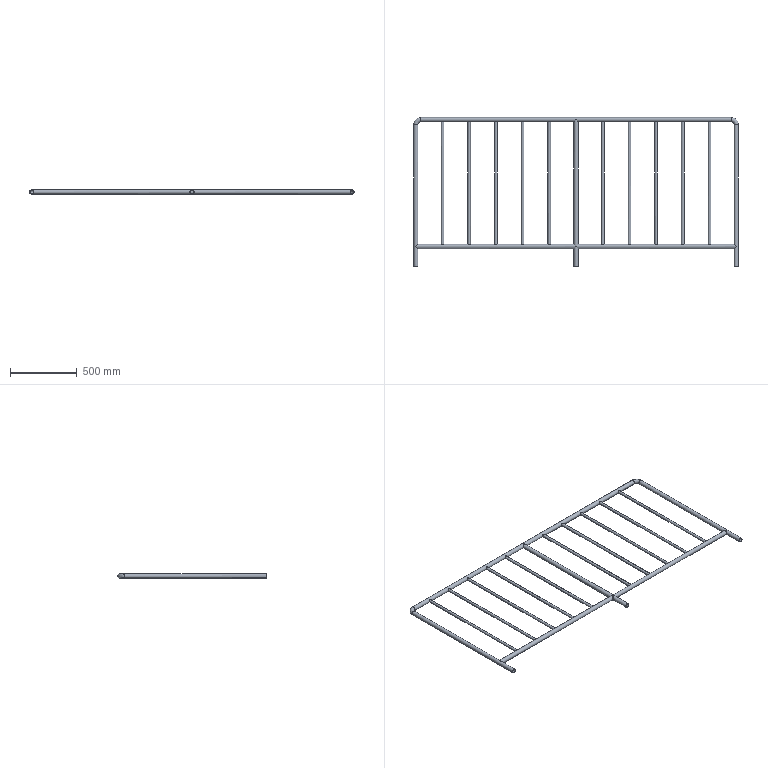Part | STEP file | PN_0002 304 guardrail 2400X1100 body-B_Default<As Machined> | 18 solids | 72 faces | box 2432 x 1116 x 32 mm | volume 2551384 mm3 | cylinder 57 | plane 11 | torus 4 | commonest cylinder face diameters 32 x31 16 x10 20 x10 28 x6